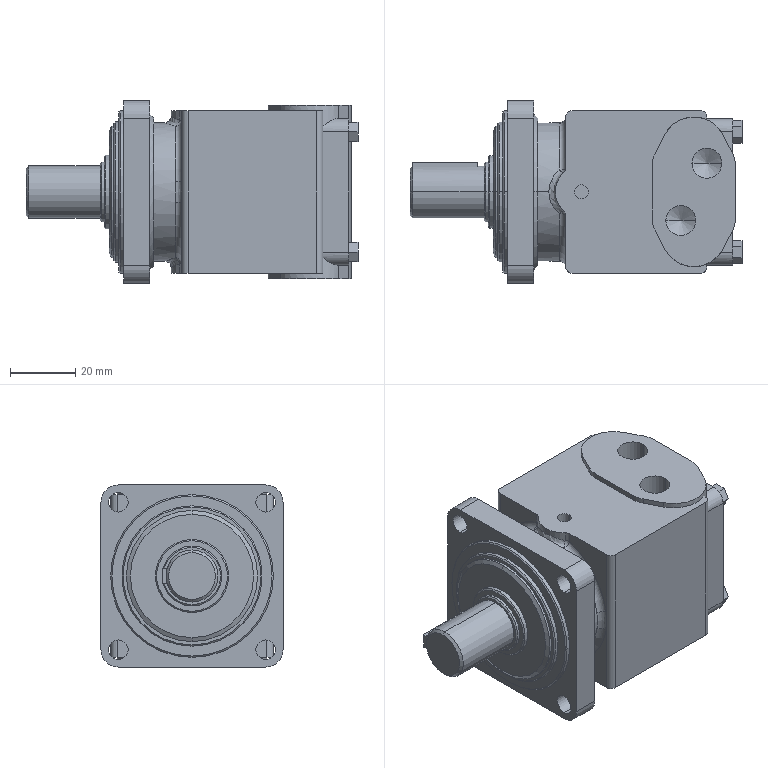Part | SolidWorks | features ICE 1, MBimport 1, Scale 1 | 1 solid | 177 faces | box 102 x 56 x 56 mm | volume 177748 mm3 | plane 79 | cylinder 64 | cone 22 | spline 4 | torus 4 | sphere 4 | commonest cylinder face diameters 16 x12 4 x8 6 x8 9.2 x8 4.28 x4 8 x4